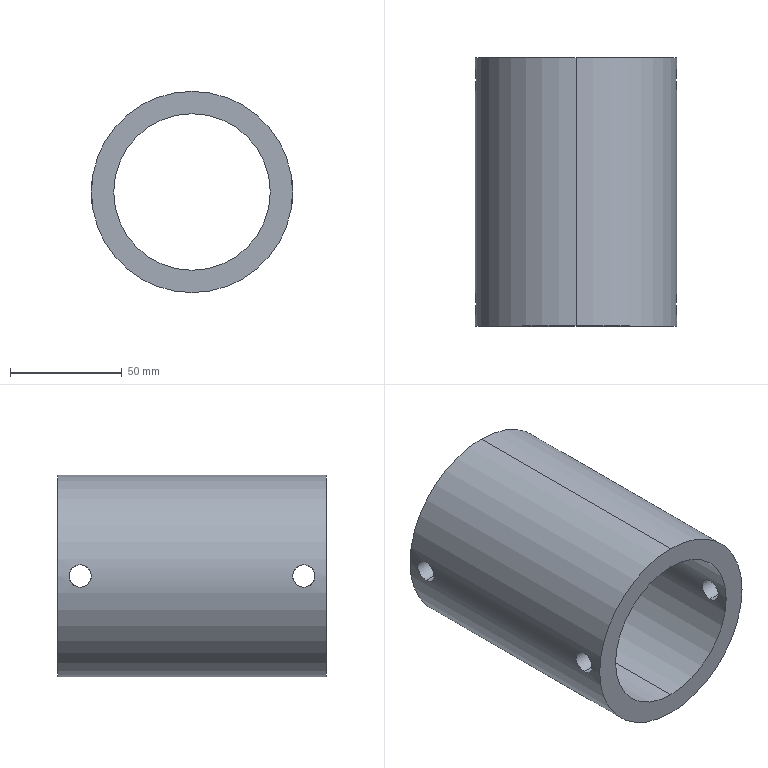Part | SolidWorks | features BaseBody 1 | 1 solid | 14 faces | box 90 x 120 x 90 mm | volume 298445 mm3 | cylinder 12 | plane 2 | commonest cylinder face diameters 10 x8 70 x2 90 x2
STEP:
#1=CARTESIAN_POINT('',(44.721,-50.,5.));
#2=VERTEX_POINT('',#1);
#3=CARTESIAN_POINT('',(44.721,-50.,-5.));
#4=VERTEX_POINT('',#3);
#5=CARTESIAN_POINT('',(44.721,-50.,5.));
#6=CARTESIAN_POINT('',(44.721,-50.33,5.));
#7=CARTESIAN_POINT('',(44.725,-50.656,4.968));
#8=CARTESIAN_POINT('',(44.735,-51.135,4.872));
#9=CARTESIAN_POINT('',(44.74,-51.294,4.833));
#10=CARTESIAN_POINT('',(44.75,-51.608,4.737));
#11=CARTESIAN_POINT('',(44.756,-51.764,4.681));
#12=CARTESIAN_POINT('',(44.775,-52.218,4.493));
#13=CARTESIAN_POINT('',(44.791,-52.505,4.34));
#14=CARTESIAN_POINT('',(44.824,-53.048,3.977));
#15=CARTESIAN_POINT('',(44.843,-53.305,3.766));
#16=CARTESIAN_POINT('',(44.879,-53.766,3.305));
#17=CARTESIAN_POINT('',(44.897,-53.973,3.053));
#18=CARTESIAN_POINT('',(44.931,-54.338,2.507));
#19=CARTESIAN_POINT('',(44.946,-54.494,2.217));
#20=CARTESIAN_POINT('',(44.972,-54.743,1.615));
#21=CARTESIAN_POINT('',(44.982,-54.839,1.3));
#22=CARTESIAN_POINT('',(44.996,-54.968,0.6537));
#23=CARTESIAN_POINT('',(45.,-55.,0.3268));
#24=CARTESIAN_POINT('',(45.,-55.,-0.3342));
#25=CARTESIAN_POINT('',(44.996,-54.967,-0.6592));
#26=CARTESIAN_POINT('',(44.986,-54.871,-1.139));
#27=CARTESIAN_POINT('',(44.982,-54.832,-1.297));
#28=CARTESIAN_POINT('',(44.971,-54.736,-1.611));
#29=CARTESIAN_POINT('',(44.966,-54.68,-1.767));
#30=CARTESIAN_POINT('',(44.946,-54.492,-2.221));
#31=CARTESIAN_POINT('',(44.931,-54.338,-2.508));
#32=CARTESIAN_POINT('',(44.897,-53.975,-3.051));
#33=CARTESIAN_POINT('',(44.879,-53.763,-3.308));
#34=CARTESIAN_POINT('',(44.843,-53.302,-3.768));
#35=CARTESIAN_POINT('',(44.824,-53.051,-3.975));
#36=CARTESIAN_POINT('',(44.791,-52.504,-4.34));
#37=CARTESIAN_POINT('',(44.775,-52.213,-4.495));
#38=CARTESIAN_POINT('',(44.749,-51.612,-4.744));
#39=CARTESIAN_POINT('',(44.739,-51.296,-4.84));
#40=CARTESIAN_POINT('',(44.725,-50.651,-4.968));
#41=CARTESIAN_POINT('',(44.721,-50.326,-5.));
#42=CARTESIAN_POINT('',(44.721,-50.,-5.));
#43=B_SPLINE_CURVE_WITH_KNOTS('',3,(#5,#6,#7,#8,#9,#10,#11,#12,#13,#14,#15,#16,#17,#18,#19,#20,#21,#22,#23,#24,#25,#26,#27,#28,#29,#30,#31,#32,#33,#34,#35,#36,#37,#38,#39,#40,#41,#42),.UNSPECIFIED.,.F.,.F.,(4,2,2,2,2,2,2,2,2,2,2,2,2,2,2,2,2,2,4),(0.02347,0.02445,0.02493,0.02542,0.0264,0.02738,0.02836,0.02933,0.03031,0.03129,0.03227,0.03275,0.03324,0.03422,0.0352,0.03618,0.03715,0.03813,0.03911),.UNSPECIFIED.);
#44=EDGE_CURVE('',#2,#4,#43,.T.);
#45=ORIENTED_EDGE('',*,*,#44,.T.);
#46=CARTESIAN_POINT('',(34.641,-50.,-5.));
#47=VERTEX_POINT('',#46);
#48=CARTESIAN_POINT('',(45.,-50.,-5.));
#49=DIRECTION('',(-1.,0.,0.));
#50=VECTOR('',#49,1000.);
#51=LINE('',#48,#50);
#52=EDGE_CURVE('',#4,#47,#51,.T.);
#53=ORIENTED_EDGE('',*,*,#52,.T.);
#54=CARTESIAN_POINT('',(34.641,-50.,5.));
#55=VERTEX_POINT('',#54);
#56=CARTESIAN_POINT('',(34.641,-50.,5.));
#57=CARTESIAN_POINT('',(34.641,-50.331,5.));
#58=CARTESIAN_POINT('',(34.646,-50.656,4.967));
#59=CARTESIAN_POINT('',(34.659,-51.136,4.872));
#60=CARTESIAN_POINT('',(34.665,-51.294,4.832));
#61=CARTESIAN_POINT('',(34.678,-51.609,4.737));
#62=CARTESIAN_POINT('',(34.686,-51.765,4.681));
#63=CARTESIAN_POINT('',(34.711,-52.219,4.493));
#64=CARTESIAN_POINT('',(34.73,-52.506,4.339));
#65=CARTESIAN_POINT('',(34.774,-53.049,3.976));
#66=CARTESIAN_POINT('',(34.798,-53.306,3.765));
#67=CARTESIAN_POINT('',(34.844,-53.767,3.304));
#68=CARTESIAN_POINT('',(34.868,-53.973,3.053));
#69=CARTESIAN_POINT('',(34.911,-54.339,2.506));
#70=CARTESIAN_POINT('',(34.931,-54.494,2.216));
#71=CARTESIAN_POINT('',(34.964,-54.743,1.614));
#72=CARTESIAN_POINT('',(34.977,-54.84,1.299));
#73=CARTESIAN_POINT('',(34.995,-54.968,0.6532));
#74=CARTESIAN_POINT('',(35.,-55.,0.3284));
#75=CARTESIAN_POINT('',(35.,-55.,-0.3247));
#76=CARTESIAN_POINT('',(34.995,-54.967,-0.6565));
#77=CARTESIAN_POINT('',(34.977,-54.84,-1.298));
#78=CARTESIAN_POINT('',(34.964,-54.745,-1.61));
#79=CARTESIAN_POINT('',(34.939,-54.557,-2.064));
#80=CARTESIAN_POINT('',(34.93,-54.486,-2.214));
#81=CARTESIAN_POINT('',(34.911,-54.331,-2.504));
#82=CARTESIAN_POINT('',(34.9,-54.247,-2.643));
#83=CARTESIAN_POINT('',(34.868,-53.976,-3.049));
#84=CARTESIAN_POINT('',(34.845,-53.769,-3.302));
#85=CARTESIAN_POINT('',(34.797,-53.303,-3.768));
#86=CARTESIAN_POINT('',(34.774,-53.051,-3.975));
#87=CARTESIAN_POINT('',(34.731,-52.509,-4.337));
#88=CARTESIAN_POINT('',(34.711,-52.217,-4.494));
#89=CARTESIAN_POINT('',(34.677,-51.612,-4.744));
#90=CARTESIAN_POINT('',(34.664,-51.3,-4.839));
#91=CARTESIAN_POINT('',(34.646,-50.658,-4.967));
#92=CARTESIAN_POINT('',(34.641,-50.327,-5.));
#93=CARTESIAN_POINT('',(34.641,-50.,-5.));
#94=B_SPLINE_CURVE_WITH_KNOTS('',3,(#56,#57,#58,#59,#60,#61,#62,#63,#64,#65,#66,#67,#68,#69,#70,#71,#72,#73,#74,#75,#76,#77,#78,#79,#80,#81,#82,#83,#84,#85,#86,#87,#88,#89,#90,#91,#92,#93),.UNSPECIFIED.,.F.,.F.,(4,2,2,2,2,2,2,2,2,2,2,2,2,2,2,2,2,2,4),(0.,0.0009783,0.001467,0.001957,0.002935,0.003913,0.004891,0.00587,0.006848,0.007826,0.008804,0.009783,0.01027,0.01076,0.01174,0.01272,0.0137,0.01467,0.01565),.UNSPECIFIED.);
#95=EDGE_CURVE('',#55,#47,#94,.T.);
#96=ORIENTED_EDGE('',*,*,#95,.F.);
#97=CARTESIAN_POINT('',(45.,-50.,5.));
#98=DIRECTION('',(-1.,0.,0.));
#99=VECTOR('',#98,1000.);
#100=LINE('',#97,#99);
#101=EDGE_CURVE('',#2,#55,#100,.T.);
#102=ORIENTED_EDGE('',*,*,#101,.F.);
#103=EDGE_LOOP('',(#45,#53,#96,#102));
#104=FACE_OUTER_BOUND('',#103,.T.);
#105=CARTESIAN_POINT('',(45.,-50.,0.));
#106=DIRECTION('',(-1.,0.,0.));
#107=DIRECTION('',(0.,0.,1.));
#108=AXIS2_PLACEMENT_3D('',#105,#106,#107);
#109=CYLINDRICAL_SURFACE('',#108,5.);
#110=ADVANCED_FACE('',(#104),#109,.F.);
#111=CARTESIAN_POINT('',(-34.641,-50.,-5.));
#112=VERTEX_POINT('',#111);
#113=CARTESIAN_POINT('',(-34.641,-50.,5.));
#114=VERTEX_POINT('',#113);
#115=CARTESIAN_POINT('',(-34.641,-50.,-5.));
#116=CARTESIAN_POINT('',(-34.641,-50.326,-5.));
#117=CARTESIAN_POINT('',(-34.646,-50.651,-4.968));
#118=CARTESIAN_POINT('',(-34.664,-51.297,-4.84));
#119=CARTESIAN_POINT('',(-34.677,-51.612,-4.744));
#120=CARTESIAN_POINT('',(-34.71,-52.214,-4.495));
#121=CARTESIAN_POINT('',(-34.73,-52.505,-4.339));
#122=CARTESIAN_POINT('',(-34.774,-53.051,-3.975));
#123=CARTESIAN_POINT('',(-34.797,-53.303,-3.768));
#124=CARTESIAN_POINT('',(-34.844,-53.764,-3.308));
#125=CARTESIAN_POINT('',(-34.868,-53.975,-3.051));
#126=CARTESIAN_POINT('',(-34.911,-54.338,-2.508));
#127=CARTESIAN_POINT('',(-34.931,-54.491,-2.222));
#128=CARTESIAN_POINT('',(-34.956,-54.68,-1.767));
#129=CARTESIAN_POINT('',(-34.963,-54.736,-1.611));
#130=CARTESIAN_POINT('',(-34.976,-54.832,-1.297));
#131=CARTESIAN_POINT('',(-34.982,-54.871,-1.139));
#132=CARTESIAN_POINT('',(-34.995,-54.967,-0.6595));
#133=CARTESIAN_POINT('',(-35.,-55.,-0.3338));
#134=CARTESIAN_POINT('',(-35.,-55.,0.3271));
#135=CARTESIAN_POINT('',(-34.995,-54.968,0.6522));
#136=CARTESIAN_POINT('',(-34.978,-54.841,1.292));
#137=CARTESIAN_POINT('',(-34.964,-54.745,1.61));
#138=CARTESIAN_POINT('',(-34.931,-54.494,2.215));
#139=CARTESIAN_POINT('',(-34.912,-54.341,2.502));
#140=CARTESIAN_POINT('',(-34.868,-53.979,3.046));
#141=CARTESIAN_POINT('',(-34.845,-53.768,3.303));
#142=CARTESIAN_POINT('',(-34.798,-53.308,3.764));
#143=CARTESIAN_POINT('',(-34.775,-53.057,3.971));
#144=CARTESIAN_POINT('',(-34.731,-52.51,4.337));
#145=CARTESIAN_POINT('',(-34.711,-52.22,4.492));
#146=CARTESIAN_POINT('',(-34.678,-51.619,4.742));
#147=CARTESIAN_POINT('',(-34.664,-51.304,4.838));
#148=CARTESIAN_POINT('',(-34.646,-50.658,4.968));
#149=CARTESIAN_POINT('',(-34.641,-50.331,5.));
#150=CARTESIAN_POINT('',(-34.641,-50.,5.));
#151=B_SPLINE_CURVE_WITH_KNOTS('',3,(#115,#116,#117,#118,#119,#120,#121,#122,#123,#124,#125,#126,#127,#128,#129,#130,#131,#132,#133,#134,#135,#136,#137,#138,#139,#140,#141,#142,#143,#144,#145,#146,#147,#148,#149,#150),.UNSPECIFIED.,.F.,.F.,(4,2,2,2,2,2,2,2,2,2,2,2,2,2,2,2,2,4),(0.01565,0.01663,0.01761,0.01859,0.01956,0.02054,0.02152,0.02201,0.0225,0.02348,0.02445,0.02543,0.02641,0.02739,0.02837,0.02934,0.03032,0.0313),.UNSPECIFIED.);
#152=EDGE_CURVE('',#112,#114,#151,.T.);
#153=ORIENTED_EDGE('',*,*,#152,.F.);
#154=CARTESIAN_POINT('',(-44.721,-50.,-5.));
#155=VERTEX_POINT('',#154);
#156=CARTESIAN_POINT('',(45.,-50.,-5.));
#157=DIRECTION('',(-1.,0.,0.));
#158=VECTOR('',#157,1000.);
#159=LINE('',#156,#158);
#160=EDGE_CURVE('',#112,#155,#159,.T.);
#161=ORIENTED_EDGE('',*,*,#160,.T.);
#162=CARTESIAN_POINT('',(-44.721,-50.,5.));
#163=VERTEX_POINT('',#162);
#164=CARTESIAN_POINT('',(-44.721,-50.,-5.));
#165=CARTESIAN_POINT('',(-44.721,-50.326,-5.));
#166=CARTESIAN_POINT('',(-44.725,-50.651,-4.968));
#167=CARTESIAN_POINT('',(-44.739,-51.296,-4.84));
#168=CARTESIAN_POINT('',(-44.749,-51.612,-4.744));
#169=CARTESIAN_POINT('',(-44.775,-52.214,-4.495));
#170=CARTESIAN_POINT('',(-44.791,-52.504,-4.34));
#171=CARTESIAN_POINT('',(-44.824,-53.051,-3.975));
#172=CARTESIAN_POINT('',(-44.843,-53.303,-3.768));
#173=CARTESIAN_POINT('',(-44.879,-53.764,-3.308));
#174=CARTESIAN_POINT('',(-44.897,-53.975,-3.051));
#175=CARTESIAN_POINT('',(-44.931,-54.338,-2.508));
#176=CARTESIAN_POINT('',(-44.946,-54.492,-2.221));
#177=CARTESIAN_POINT('',(-44.966,-54.68,-1.767));
#178=CARTESIAN_POINT('',(-44.971,-54.736,-1.611));
#179=CARTESIAN_POINT('',(-44.982,-54.832,-1.297));
#180=CARTESIAN_POINT('',(-44.986,-54.871,-1.138));
#181=CARTESIAN_POINT('',(-44.996,-54.967,-0.6591));
#182=CARTESIAN_POINT('',(-45.,-55.,-0.3342));
#183=CARTESIAN_POINT('',(-45.,-55.,0.3267));
#184=CARTESIAN_POINT('',(-44.996,-54.968,0.652));
#185=CARTESIAN_POINT('',(-44.986,-54.873,1.132));
#186=CARTESIAN_POINT('',(-44.982,-54.834,1.29));
#187=CARTESIAN_POINT('',(-44.972,-54.738,1.604));
#188=CARTESIAN_POINT('',(-44.966,-54.683,1.76));
#189=CARTESIAN_POINT('',(-44.946,-54.495,2.215));
#190=CARTESIAN_POINT('',(-44.931,-54.341,2.502));
#191=CARTESIAN_POINT('',(-44.898,-53.979,3.045));
#192=CARTESIAN_POINT('',(-44.879,-53.768,3.303));
#193=CARTESIAN_POINT('',(-44.843,-53.308,3.764));
#194=CARTESIAN_POINT('',(-44.825,-53.056,3.971));
#195=CARTESIAN_POINT('',(-44.791,-52.51,4.337));
#196=CARTESIAN_POINT('',(-44.775,-52.22,4.492));
#197=CARTESIAN_POINT('',(-44.75,-51.619,4.742));
#198=CARTESIAN_POINT('',(-44.739,-51.304,4.838));
#199=CARTESIAN_POINT('',(-44.725,-50.657,4.968));
#200=CARTESIAN_POINT('',(-44.721,-50.331,5.));
#201=CARTESIAN_POINT('',(-44.721,-50.,5.));
#202=B_SPLINE_CURVE_WITH_KNOTS('',3,(#164,#165,#166,#167,#168,#169,#170,#171,#172,#173,#174,#175,#176,#177,#178,#179,#180,#181,#182,#183,#184,#185,#186,#187,#188,#189,#190,#191,#192,#193,#194,#195,#196,#197,#198,#199,#200,#201),.UNSPECIFIED.,.F.,.F.,(4,2,2,2,2,2,2,2,2,2,2,2,2,2,2,2,2,2,4),(0.01564,0.01662,0.0176,0.01858,0.01955,0.02053,0.02151,0.022,0.02249,0.02346,0.02444,0.02493,0.02542,0.0264,0.02737,0.02835,0.02933,0.03031,0.03128),.UNSPECIFIED.);
#203=EDGE_CURVE('',#155,#163,#202,.T.);
#204=ORIENTED_EDGE('',*,*,#203,.T.);
#205=CARTESIAN_POINT('',(45.,-50.,5.));
#206=DIRECTION('',(-1.,0.,0.));
#207=VECTOR('',#206,1000.);
#208=LINE('',#205,#207);
#209=EDGE_CURVE('',#114,#163,#208,.T.);
#210=ORIENTED_EDGE('',*,*,#209,.F.);
#211=EDGE_LOOP('',(#153,#161,#204,#210));
#212=FACE_OUTER_BOUND('',#211,.T.);
#213=CARTESIAN_POINT('',(45.,-50.,0.));
#214=DIRECTION('',(-1.,0.,0.));
#215=DIRECTION('',(0.,0.,1.));
#216=AXIS2_PLACEMENT_3D('',#213,#214,#215);
#217=CYLINDRICAL_SURFACE('',#216,5.);
#218=ADVANCED_FACE('',(#212),#217,.F.);
#219=CARTESIAN_POINT('',(44.721,50.,-5.));
#220=VERTEX_POINT('',#219);
#221=CARTESIAN_POINT('',(44.721,50.,5.));
#222=VERTEX_POINT('',#221);
#223=CARTESIAN_POINT('',(44.721,50.,-5.));
#224=CARTESIAN_POINT('',(44.721,49.67,-5.));
#225=CARTESIAN_POINT('',(44.725,49.344,-4.968));
#226=CARTESIAN_POINT('',(44.735,48.865,-4.872));
#227=CARTESIAN_POINT('',(44.74,48.706,-4.833));
#228=CARTESIAN_POINT('',(44.75,48.392,-4.737));
#229=CARTESIAN_POINT('',(44.756,48.236,-4.681));
#230=CARTESIAN_POINT('',(44.775,47.782,-4.493));
#231=CARTESIAN_POINT('',(44.791,47.495,-4.34));
#232=CARTESIAN_POINT('',(44.824,46.952,-3.977));
#233=CARTESIAN_POINT('',(44.843,46.695,-3.766));
#234=CARTESIAN_POINT('',(44.879,46.234,-3.305));
#235=CARTESIAN_POINT('',(44.897,46.027,-3.053));
#236=CARTESIAN_POINT('',(44.931,45.662,-2.507));
#237=CARTESIAN_POINT('',(44.946,45.506,-2.217));
#238=CARTESIAN_POINT('',(44.972,45.257,-1.615));
#239=CARTESIAN_POINT('',(44.982,45.161,-1.3));
#240=CARTESIAN_POINT('',(44.996,45.032,-0.6537));
#241=CARTESIAN_POINT('',(45.,45.,-0.3268));
#242=CARTESIAN_POINT('',(45.,45.,0.3342));
#243=CARTESIAN_POINT('',(44.996,45.033,0.6592));
#244=CARTESIAN_POINT('',(44.986,45.129,1.139));
#245=CARTESIAN_POINT('',(44.982,45.168,1.297));
#246=CARTESIAN_POINT('',(44.971,45.264,1.611));
#247=CARTESIAN_POINT('',(44.966,45.32,1.767));
#248=CARTESIAN_POINT('',(44.946,45.508,2.221));
#249=CARTESIAN_POINT('',(44.931,45.662,2.508));
#250=CARTESIAN_POINT('',(44.897,46.025,3.051));
#251=CARTESIAN_POINT('',(44.879,46.237,3.308));
#252=CARTESIAN_POINT('',(44.843,46.698,3.768));
#253=CARTESIAN_POINT('',(44.824,46.949,3.975));
#254=CARTESIAN_POINT('',(44.791,47.496,4.34));
#255=CARTESIAN_POINT('',(44.775,47.787,4.495));
#256=CARTESIAN_POINT('',(44.749,48.388,4.744));
#257=CARTESIAN_POINT('',(44.739,48.704,4.84));
#258=CARTESIAN_POINT('',(44.725,49.349,4.968));
#259=CARTESIAN_POINT('',(44.721,49.674,5.));
#260=CARTESIAN_POINT('',(44.721,50.,5.));
#261=B_SPLINE_CURVE_WITH_KNOTS('',3,(#223,#224,#225,#226,#227,#228,#229,#230,#231,#232,#233,#234,#235,#236,#237,#238,#239,#240,#241,#242,#243,#244,#245,#246,#247,#248,#249,#250,#251,#252,#253,#254,#255,#256,#257,#258,#259,#260),.UNSPECIFIED.,.F.,.F.,(4,2,2,2,2,2,2,2,2,2,2,2,2,2,2,2,2,2,4),(0.02347,0.02445,0.02493,0.02542,0.0264,0.02738,0.02836,0.02933,0.03031,0.03129,0.03227,0.03275,0.03324,0.03422,0.0352,0.03618,0.03715,0.03813,0.03911),.UNSPECIFIED.);
#262=EDGE_CURVE('',#220,#222,#261,.T.);
#263=ORIENTED_EDGE('',*,*,#262,.F.);
#264=CARTESIAN_POINT('',(34.641,50.,-5.));
#265=VERTEX_POINT('',#264);
#266=CARTESIAN_POINT('',(45.,50.,-5.));
#267=DIRECTION('',(-1.,0.,0.));
#268=VECTOR('',#267,1000.);
#269=LINE('',#266,#268);
#270=EDGE_CURVE('',#220,#265,#269,.T.);
#271=ORIENTED_EDGE('',*,*,#270,.T.);
#272=CARTESIAN_POINT('',(34.641,50.,5.));
#273=VERTEX_POINT('',#272);
#274=CARTESIAN_POINT('',(34.641,50.,-5.));
#275=CARTESIAN_POINT('',(34.641,49.674,-5.));
#276=CARTESIAN_POINT('',(34.646,49.349,-4.968));
#277=CARTESIAN_POINT('',(34.664,48.703,-4.84));
#278=CARTESIAN_POINT('',(34.677,48.388,-4.744));
#279=CARTESIAN_POINT('',(34.71,47.786,-4.495));
#280=CARTESIAN_POINT('',(34.73,47.495,-4.339));
#281=CARTESIAN_POINT('',(34.774,46.949,-3.975));
#282=CARTESIAN_POINT('',(34.797,46.697,-3.768));
#283=CARTESIAN_POINT('',(34.844,46.236,-3.308));
#284=CARTESIAN_POINT('',(34.868,46.025,-3.051));
#285=CARTESIAN_POINT('',(34.911,45.662,-2.508));
#286=CARTESIAN_POINT('',(34.931,45.509,-2.222));
#287=CARTESIAN_POINT('',(34.956,45.32,-1.767));
#288=CARTESIAN_POINT('',(34.963,45.264,-1.611));
#289=CARTESIAN_POINT('',(34.976,45.168,-1.297));
#290=CARTESIAN_POINT('',(34.982,45.129,-1.139));
#291=CARTESIAN_POINT('',(34.995,45.033,-0.6595));
#292=CARTESIAN_POINT('',(35.,45.,-0.3338));
#293=CARTESIAN_POINT('',(35.,45.,0.3271));
#294=CARTESIAN_POINT('',(34.995,45.032,0.6522));
#295=CARTESIAN_POINT('',(34.978,45.159,1.292));
#296=CARTESIAN_POINT('',(34.964,45.255,1.61));
#297=CARTESIAN_POINT('',(34.931,45.506,2.215));
#298=CARTESIAN_POINT('',(34.912,45.659,2.502));
#299=CARTESIAN_POINT('',(34.868,46.021,3.046));
#300=CARTESIAN_POINT('',(34.845,46.232,3.303));
#301=CARTESIAN_POINT('',(34.798,46.692,3.764));
#302=CARTESIAN_POINT('',(34.775,46.943,3.971));
#303=CARTESIAN_POINT('',(34.731,47.49,4.337));
#304=CARTESIAN_POINT('',(34.711,47.78,4.492));
#305=CARTESIAN_POINT('',(34.678,48.381,4.742));
#306=CARTESIAN_POINT('',(34.664,48.696,4.838));
#307=CARTESIAN_POINT('',(34.646,49.342,4.968));
#308=CARTESIAN_POINT('',(34.641,49.669,5.));
#309=CARTESIAN_POINT('',(34.641,50.,5.));
#310=B_SPLINE_CURVE_WITH_KNOTS('',3,(#274,#275,#276,#277,#278,#279,#280,#281,#282,#283,#284,#285,#286,#287,#288,#289,#290,#291,#292,#293,#294,#295,#296,#297,#298,#299,#300,#301,#302,#303,#304,#305,#306,#307,#308,#309),.UNSPECIFIED.,.F.,.F.,(4,2,2,2,2,2,2,2,2,2,2,2,2,2,2,2,2,4),(0.01565,0.01663,0.01761,0.01859,0.01956,0.02054,0.02152,0.02201,0.0225,0.02348,0.02445,0.02543,0.02641,0.02739,0.02837,0.02934,0.03032,0.0313),.UNSPECIFIED.);
#311=EDGE_CURVE('',#265,#273,#310,.T.);
#312=ORIENTED_EDGE('',*,*,#311,.T.);
#313=CARTESIAN_POINT('',(45.,50.,5.));
#314=DIRECTION('',(-1.,0.,0.));
#315=VECTOR('',#314,1000.);
#316=LINE('',#313,#315);
#317=EDGE_CURVE('',#222,#273,#316,.T.);
#318=ORIENTED_EDGE('',*,*,#317,.F.);
#319=EDGE_LOOP('',(#263,#271,#312,#318));
#320=FACE_OUTER_BOUND('',#319,.T.);
#321=CARTESIAN_POINT('',(45.,50.,0.));
#322=DIRECTION('',(-1.,0.,0.));
#323=DIRECTION('',(0.,0.,1.));
#324=AXIS2_PLACEMENT_3D('',#321,#322,#323);
#325=CYLINDRICAL_SURFACE('',#324,5.);
#326=ADVANCED_FACE('',(#320),#325,.F.);
#327=CARTESIAN_POINT('',(-34.641,50.,5.));
#328=VERTEX_POINT('',#327);
#329=CARTESIAN_POINT('',(-34.641,50.,-5.));
#330=VERTEX_POINT('',#329);
#331=CARTESIAN_POINT('',(-34.641,50.,5.));
#332=CARTESIAN_POINT('',(-34.641,49.669,5.));
#333=CARTESIAN_POINT('',(-34.646,49.344,4.967));
#334=CARTESIAN_POINT('',(-34.659,48.864,4.872));
#335=CARTESIAN_POINT('',(-34.665,48.706,4.832));
#336=CARTESIAN_POINT('',(-34.678,48.391,4.737));
#337=CARTESIAN_POINT('',(-34.686,48.235,4.681));
#338=CARTESIAN_POINT('',(-34.711,47.781,4.493));
#339=CARTESIAN_POINT('',(-34.73,47.494,4.339));
#340=CARTESIAN_POINT('',(-34.774,46.951,3.976));
#341=CARTESIAN_POINT('',(-34.798,46.694,3.765));
#342=CARTESIAN_POINT('',(-34.844,46.233,3.304));
#343=CARTESIAN_POINT('',(-34.868,46.027,3.053));
#344=CARTESIAN_POINT('',(-34.911,45.661,2.506));
#345=CARTESIAN_POINT('',(-34.931,45.506,2.216));
#346=CARTESIAN_POINT('',(-34.964,45.257,1.614));
#347=CARTESIAN_POINT('',(-34.977,45.16,1.299));
#348=CARTESIAN_POINT('',(-34.995,45.032,0.6532));
#349=CARTESIAN_POINT('',(-35.,45.,0.3284));
#350=CARTESIAN_POINT('',(-35.,45.,-0.3247));
#351=CARTESIAN_POINT('',(-34.995,45.033,-0.6565));
#352=CARTESIAN_POINT('',(-34.977,45.16,-1.298));
#353=CARTESIAN_POINT('',(-34.964,45.255,-1.61));
#354=CARTESIAN_POINT('',(-34.939,45.443,-2.064));
#355=CARTESIAN_POINT('',(-34.93,45.514,-2.214));
#356=CARTESIAN_POINT('',(-34.911,45.669,-2.504));
#357=CARTESIAN_POINT('',(-34.9,45.753,-2.643));
#358=CARTESIAN_POINT('',(-34.868,46.024,-3.049));
#359=CARTESIAN_POINT('',(-34.845,46.231,-3.302));
#360=CARTESIAN_POINT('',(-34.797,46.697,-3.768));
#361=CARTESIAN_POINT('',(-34.774,46.949,-3.975));
#362=CARTESIAN_POINT('',(-34.731,47.491,-4.337));
#363=CARTESIAN_POINT('',(-34.711,47.783,-4.494));
#364=CARTESIAN_POINT('',(-34.677,48.388,-4.744));
#365=CARTESIAN_POINT('',(-34.664,48.7,-4.839));
#366=CARTESIAN_POINT('',(-34.646,49.342,-4.967));
#367=CARTESIAN_POINT('',(-34.641,49.673,-5.));
#368=CARTESIAN_POINT('',(-34.641,50.,-5.));
#369=B_SPLINE_CURVE_WITH_KNOTS('',3,(#331,#332,#333,#334,#335,#336,#337,#338,#339,#340,#341,#342,#343,#344,#345,#346,#347,#348,#349,#350,#351,#352,#353,#354,#355,#356,#357,#358,#359,#360,#361,#362,#363,#364,#365,#366,#367,#368),.UNSPECIFIED.,.F.,.F.,(4,2,2,2,2,2,2,2,2,2,2,2,2,2,2,2,2,2,4),(0.,0.0009783,0.001467,0.001957,0.002935,0.003913,0.004891,0.00587,0.006848,0.007826,0.008804,0.009783,0.01027,0.01076,0.01174,0.01272,0.0137,0.01467,0.01565),.UNSPECIFIED.);
#370=EDGE_CURVE('',#328,#330,#369,.T.);
#371=ORIENTED_EDGE('',*,*,#370,.T.);
#372=CARTESIAN_POINT('',(-44.721,50.,-5.));
#373=VERTEX_POINT('',#372);
#374=CARTESIAN_POINT('',(45.,50.,-5.));
#375=DIRECTION('',(-1.,0.,0.));
#376=VECTOR('',#375,1000.);
#377=LINE('',#374,#376);
#378=EDGE_CURVE('',#330,#373,#377,.T.);
#379=ORIENTED_EDGE('',*,*,#378,.T.);
#380=CARTESIAN_POINT('',(-44.721,50.,5.));
#381=VERTEX_POINT('',#380);
#382=CARTESIAN_POINT('',(-44.721,50.,5.));
#383=CARTESIAN_POINT('',(-44.721,49.669,5.));
#384=CARTESIAN_POINT('',(-44.725,49.344,4.968));
#385=CARTESIAN_POINT('',(-44.735,48.865,4.872));
#386=CARTESIAN_POINT('',(-44.74,48.706,4.833));
#387=CARTESIAN_POINT('',(-44.75,48.392,4.737));
#388=CARTESIAN_POINT('',(-44.756,48.236,4.681));
#389=CARTESIAN_POINT('',(-44.775,47.782,4.493));
#390=CARTESIAN_POINT('',(-44.791,47.495,4.339));
#391=CARTESIAN_POINT('',(-44.824,46.951,3.976));
#392=CARTESIAN_POINT('',(-44.843,46.694,3.765));
#393=CARTESIAN_POINT('',(-44.879,46.233,3.304));
#394=CARTESIAN_POINT('',(-44.897,46.026,3.053));
#395=CARTESIAN_POINT('',(-44.931,45.661,2.506));
#396=CARTESIAN_POINT('',(-44.946,45.506,2.215));
#397=CARTESIAN_POINT('',(-44.972,45.256,1.614));
#398=CARTESIAN_POINT('',(-44.982,45.16,1.298));
#399=CARTESIAN_POINT('',(-44.996,45.032,0.6528));
#400=CARTESIAN_POINT('',(-45.,45.,0.3282));
#401=CARTESIAN_POINT('',(-45.,45.,-0.3246));
#402=CARTESIAN_POINT('',(-44.996,45.032,-0.6561));
#403=CARTESIAN_POINT('',(-44.982,45.16,-1.298));
#404=CARTESIAN_POINT('',(-44.972,45.255,-1.609));
#405=CARTESIAN_POINT('',(-44.953,45.443,-2.064));
#406=CARTESIAN_POINT('',(-44.946,45.514,-2.214));
#407=CARTESIAN_POINT('',(-44.931,45.668,-2.503));
#408=CARTESIAN_POINT('',(-44.923,45.753,-2.643));
#409=CARTESIAN_POINT('',(-44.897,46.024,-3.049));
#410=CARTESIAN_POINT('',(-44.879,46.231,-3.302));
#411=CARTESIAN_POINT('',(-44.843,46.697,-3.768));
#412=CARTESIAN_POINT('',(-44.824,46.95,-3.975));
#413=CARTESIAN_POINT('',(-44.799,47.356,-4.247));
#414=CARTESIAN_POINT('',(-44.791,47.496,-4.331));
#415=CARTESIAN_POINT('',(-44.776,47.785,-4.486));
#416=CARTESIAN_POINT('',(-44.769,47.935,-4.557));
#417=CARTESIAN_POINT('',(-44.749,48.389,-4.745));
#418=CARTESIAN_POINT('',(-44.739,48.701,-4.839));
#419=CARTESIAN_POINT('',(-44.725,49.342,-4.967));
#420=CARTESIAN_POINT('',(-44.721,49.674,-5.));
#421=CARTESIAN_POINT('',(-44.721,50.,-5.));
#422=B_SPLINE_CURVE_WITH_KNOTS('',3,(#382,#383,#384,#385,#386,#387,#388,#389,#390,#391,#392,#393,#394,#395,#396,#397,#398,#399,#400,#401,#402,#403,#404,#405,#406,#407,#408,#409,#410,#411,#412,#413,#414,#415,#416,#417,#418,#419,#420,#421),.UNSPECIFIED.,.F.,.F.,(4,2,2,2,2,2,2,2,2,2,2,2,2,2,2,2,2,2,2,4),(0.,0.0009778,0.001467,0.001956,0.002933,0.003911,0.004889,0.005867,0.006844,0.007822,0.0088,0.009778,0.01027,0.01076,0.01173,0.01271,0.0132,0.01369,0.01467,0.01564),.UNSPECIFIED.);
#423=EDGE_CURVE('',#381,#373,#422,.T.);
#424=ORIENTED_EDGE('',*,*,#423,.F.);
#425=CARTESIAN_POINT('',(45.,50.,5.));
#426=DIRECTION('',(-1.,0.,0.));
#427=VECTOR('',#426,1000.);
#428=LINE('',#425,#427);
#429=EDGE_CURVE('',#328,#381,#428,.T.);
#430=ORIENTED_EDGE('',*,*,#429,.F.);
#431=EDGE_LOOP('',(#371,#379,#424,#430));
#432=FACE_OUTER_BOUND('',#431,.T.);
#433=CARTESIAN_POINT('',(45.,50.,0.));
#434=DIRECTION('',(-1.,0.,0.));
#435=DIRECTION('',(0.,0.,1.));
#436=AXIS2_PLACEMENT_3D('',#433,#434,#435);
#437=CYLINDRICAL_SURFACE('',#436,5.);
#438=ADVANCED_FACE('',(#432),#437,.F.);
#439=ORIENTED_EDGE('',*,*,#370,.F.);
#440=CARTESIAN_POINT('',(-34.641,50.,-5.));
#441=CARTESIAN_POINT('',(-34.641,50.326,-5.));
#442=CARTESIAN_POINT('',(-34.646,50.651,-4.968));
#443=CARTESIAN_POINT('',(-34.664,51.297,-4.84));
#444=CARTESIAN_POINT('',(-34.677,51.612,-4.744));
#445=CARTESIAN_POINT('',(-34.71,52.214,-4.495));
#446=CARTESIAN_POINT('',(-34.73,52.505,-4.339));
#447=CARTESIAN_POINT('',(-34.774,53.051,-3.975));
#448=CARTESIAN_POINT('',(-34.797,53.303,-3.768));
#449=CARTESIAN_POINT('',(-34.844,53.764,-3.308));
#450=CARTESIAN_POINT('',(-34.868,53.975,-3.051));
#451=CARTESIAN_POINT('',(-34.911,54.338,-2.508));
#452=CARTESIAN_POINT('',(-34.931,54.491,-2.222));
#453=CARTESIAN_POINT('',(-34.956,54.68,-1.767));
#454=CARTESIAN_POINT('',(-34.963,54.736,-1.611));
#455=CARTESIAN_POINT('',(-34.976,54.832,-1.297));
#456=CARTESIAN_POINT('',(-34.982,54.871,-1.139));
#457=CARTESIAN_POINT('',(-34.995,54.967,-0.6595));
#458=CARTESIAN_POINT('',(-35.,55.,-0.3338));
#459=CARTESIAN_POINT('',(-35.,55.,0.3271));
#460=CARTESIAN_POINT('',(-34.995,54.968,0.6522));
#461=CARTESIAN_POINT('',(-34.978,54.841,1.292));
#462=CARTESIAN_POINT('',(-34.964,54.745,1.61));
#463=CARTESIAN_POINT('',(-34.931,54.494,2.215));
#464=CARTESIAN_POINT('',(-34.912,54.341,2.502));
#465=CARTESIAN_POINT('',(-34.868,53.979,3.046));
#466=CARTESIAN_POINT('',(-34.845,53.768,3.303));
#467=CARTESIAN_POINT('',(-34.798,53.308,3.764));
#468=CARTESIAN_POINT('',(-34.775,53.057,3.971));
#469=CARTESIAN_POINT('',(-34.731,52.51,4.337));
#470=CARTESIAN_POINT('',(-34.711,52.22,4.492));
#471=CARTESIAN_POINT('',(-34.678,51.619,4.742));
#472=CARTESIAN_POINT('',(-34.664,51.304,4.838));
#473=CARTESIAN_POINT('',(-34.646,50.658,4.968));
#474=CARTESIAN_POINT('',(-34.641,50.331,5.));
#475=CARTESIAN_POINT('',(-34.641,50.,5.));
#476=B_SPLINE_CURVE_WITH_KNOTS('',3,(#440,#441,#442,#443,#444,#445,#446,#447,#448,#449,#450,#451,#452,#453,#454,#455,#456,#457,#458,#459,#460,#461,#462,#463,#464,#465,#466,#467,#468,#469,#470,#471,#472,#473,#474,#475),.UNSPECIFIED.,.F.,.F.,(4,2,2,2,2,2,2,2,2,2,2,2,2,2,2,2,2,4),(0.01565,0.01663,0.01761,0.01859,0.01956,0.02054,0.02152,0.02201,0.0225,0.02348,0.02445,0.02543,0.02641,0.02739,0.02837,0.02934,0.03032,0.0313),.UNSPECIFIED.);
#477=EDGE_CURVE('',#330,#328,#476,.T.);
#478=ORIENTED_EDGE('',*,*,#477,.F.);
#479=EDGE_LOOP('',(#439,#478));
#480=FACE_BOUND('',#479,.T.);
#481=CARTESIAN_POINT('',(-34.641,-50.,5.));
#482=CARTESIAN_POINT('',(-34.641,-49.669,5.));
#483=CARTESIAN_POINT('',(-34.646,-49.344,4.967));
#484=CARTESIAN_POINT('',(-34.659,-48.864,4.872));
#485=CARTESIAN_POINT('',(-34.665,-48.706,4.832));
#486=CARTESIAN_POINT('',(-34.678,-48.391,4.737));
#487=CARTESIAN_POINT('',(-34.686,-48.235,4.681));
#488=CARTESIAN_POINT('',(-34.711,-47.781,4.493));
#489=CARTESIAN_POINT('',(-34.73,-47.494,4.339));
#490=CARTESIAN_POINT('',(-34.774,-46.951,3.976));
#491=CARTESIAN_POINT('',(-34.798,-46.694,3.765));
#492=CARTESIAN_POINT('',(-34.844,-46.233,3.304));
#493=CARTESIAN_POINT('',(-34.868,-46.027,3.053));
#494=CARTESIAN_POINT('',(-34.911,-45.661,2.506));
#495=CARTESIAN_POINT('',(-34.931,-45.506,2.216));
#496=CARTESIAN_POINT('',(-34.964,-45.257,1.614));
#497=CARTESIAN_POINT('',(-34.977,-45.16,1.299));
#498=CARTESIAN_POINT('',(-34.995,-45.032,0.6532));
#499=CARTESIAN_POINT('',(-35.,-45.,0.3284));
#500=CARTESIAN_POINT('',(-35.,-45.,-0.3247));
#501=CARTESIAN_POINT('',(-34.995,-45.033,-0.6565));
#502=CARTESIAN_POINT('',(-34.977,-45.16,-1.298));
#503=CARTESIAN_POINT('',(-34.964,-45.255,-1.61));
#504=CARTESIAN_POINT('',(-34.939,-45.443,-2.064));
#505=CARTESIAN_POINT('',(-34.93,-45.514,-2.214));
#506=CARTESIAN_POINT('',(-34.911,-45.669,-2.504));
#507=CARTESIAN_POINT('',(-34.9,-45.753,-2.643));
#508=CARTESIAN_POINT('',(-34.868,-46.024,-3.049));
#509=CARTESIAN_POINT('',(-34.845,-46.231,-3.302));
#510=CARTESIAN_POINT('',(-34.797,-46.697,-3.768));
#511=CARTESIAN_POINT('',(-34.774,-46.949,-3.975));
#512=CARTESIAN_POINT('',(-34.731,-47.491,-4.337));
#513=CARTESIAN_POINT('',(-34.711,-47.783,-4.494));
#514=CARTESIAN_POINT('',(-34.677,-48.388,-4.744));
#515=CARTESIAN_POINT('',(-34.664,-48.7,-4.839));
#516=CARTESIAN_POINT('',(-34.646,-49.342,-4.967));
#517=CARTESIAN_POINT('',(-34.641,-49.673,-5.));
#518=CARTESIAN_POINT('',(-34.641,-50.,-5.));
#519=B_SPLINE_CURVE_WITH_KNOTS('',3,(#481,#482,#483,#484,#485,#486,#487,#488,#489,#490,#491,#492,#493,#494,#495,#496,#497,#498,#499,#500,#501,#502,#503,#504,#505,#506,#507,#508,#509,#510,#511,#512,#513,#514,#515,#516,#517,#518),.UNSPECIFIED.,.F.,.F.,(4,2,2,2,2,2,2,2,2,2,2,2,2,2,2,2,2,2,4),(0.,0.0009783,0.001467,0.001957,0.002935,0.003913,0.004891,0.00587,0.006848,0.007826,0.008804,0.009783,0.01027,0.01076,0.01174,0.01272,0.0137,0.01467,0.01565),.UNSPECIFIED.);
#520=EDGE_CURVE('',#114,#112,#519,.T.);
#521=ORIENTED_EDGE('',*,*,#520,.T.);
#522=ORIENTED_EDGE('',*,*,#152,.T.);
#523=EDGE_LOOP('',(#521,#522));
#524=FACE_BOUND('',#523,.T.);
#525=CARTESIAN_POINT('',(0.,60.,-35.));
#526=VERTEX_POINT('',#525);
#527=CARTESIAN_POINT('',(0.,60.,35.));
#528=VERTEX_POINT('',#527);
#529=CARTESIAN_POINT('',(0.,60.,0.));
#530=DIRECTION('',(0.,1.,0.));
#531=DIRECTION('',(0.,0.,1.));
#532=AXIS2_PLACEMENT_3D('',#529,#530,#531);
#533=CIRCLE('',#532,35.);
#534=EDGE_CURVE('',#526,#528,#533,.T.);
#535=ORIENTED_EDGE('',*,*,#534,.T.);
#536=CARTESIAN_POINT('',(0.,-60.,35.));
#537=VERTEX_POINT('',#536);
#538=CARTESIAN_POINT('',(0.,60.,35.));
#539=DIRECTION('',(0.,-1.,0.));
#540=VECTOR('',#539,1000.);
#541=LINE('',#538,#540);
#542=EDGE_CURVE('',#528,#537,#541,.T.);
#543=ORIENTED_EDGE('',*,*,#542,.T.);
#544=CARTESIAN_POINT('',(0.,-60.,-35.));
#545=VERTEX_POINT('',#544);
#546=CARTESIAN_POINT('',(0.,-60.,0.));
#547=DIRECTION('',(0.,1.,0.));
#548=DIRECTION('',(0.,0.,1.));
#549=AXIS2_PLACEMENT_3D('',#546,#547,#548);
#550=CIRCLE('',#549,35.);
#551=EDGE_CURVE('',#545,#537,#550,.T.);
#552=ORIENTED_EDGE('',*,*,#551,.F.);
#553=CARTESIAN_POINT('',(0.,60.,-35.));
#554=DIRECTION('',(0.,-1.,0.));
#555=VECTOR('',#554,1000.);
#556=LINE('',#553,#555);
#557=EDGE_CURVE('',#526,#545,#556,.T.);
#558=ORIENTED_EDGE('',*,*,#557,.F.);
#559=EDGE_LOOP('',(#535,#543,#552,#558));
#560=FACE_OUTER_BOUND('',#559,.T.);
#561=CARTESIAN_POINT('',(0.,60.,0.));
#562=DIRECTION('',(0.,-1.,0.));
#563=DIRECTION('',(0.,0.,-1.));
#564=AXIS2_PLACEMENT_3D('',#561,#562,#563);
#565=CYLINDRICAL_SURFACE('',#564,35.);
#566=ADVANCED_FACE('',(#480,#524,#560),#565,.F.);
#567=ORIENTED_EDGE('',*,*,#44,.F.);
#568=CARTESIAN_POINT('',(44.721,-50.,-5.));
#569=CARTESIAN_POINT('',(44.721,-49.674,-5.));
#570=CARTESIAN_POINT('',(44.725,-49.342,-4.967));
#571=CARTESIAN_POINT('',(44.739,-48.701,-4.839));
#572=CARTESIAN_POINT('',(44.749,-48.389,-4.745));
#573=CARTESIAN_POINT('',(44.769,-47.935,-4.556));
#574=CARTESIAN_POINT('',(44.776,-47.785,-4.485));
#575=CARTESIAN_POINT('',(44.791,-47.495,-4.331));
#576=CARTESIAN_POINT('',(44.799,-47.355,-4.247));
#577=CARTESIAN_POINT('',(44.824,-46.949,-3.975));
#578=CARTESIAN_POINT('',(44.843,-46.697,-3.768));
#579=CARTESIAN_POINT('',(44.879,-46.23,-3.301));
#580=CARTESIAN_POINT('',(44.897,-46.024,-3.049));
#581=CARTESIAN_POINT('',(44.923,-45.752,-2.643));
#582=CARTESIAN_POINT('',(44.931,-45.668,-2.503));
#583=CARTESIAN_POINT('',(44.946,-45.514,-2.213));
#584=CARTESIAN_POINT('',(44.953,-45.443,-2.063));
#585=CARTESIAN_POINT('',(44.972,-45.255,-1.609));
#586=CARTESIAN_POINT('',(44.982,-45.16,-1.298));
#587=CARTESIAN_POINT('',(44.996,-45.032,-0.6562));
#588=CARTESIAN_POINT('',(45.,-45.,-0.3246));
#589=CARTESIAN_POINT('',(45.,-45.,0.3283));
#590=CARTESIAN_POINT('',(44.996,-45.032,0.6529));
#591=CARTESIAN_POINT('',(44.982,-45.16,1.298));
#592=CARTESIAN_POINT('',(44.972,-45.256,1.614));
#593=CARTESIAN_POINT('',(44.946,-45.506,2.216));
#594=CARTESIAN_POINT('',(44.931,-45.661,2.507));
#595=CARTESIAN_POINT('',(44.897,-46.027,3.053));
#596=CARTESIAN_POINT('',(44.879,-46.234,3.305));
#597=CARTESIAN_POINT('',(44.843,-46.694,3.766));
#598=CARTESIAN_POINT('',(44.824,-46.952,3.977));
#599=CARTESIAN_POINT('',(44.791,-47.495,4.339));
#600=CARTESIAN_POINT('',(44.775,-47.782,4.493));
#601=CARTESIAN_POINT('',(44.756,-48.236,4.681));
#602=CARTESIAN_POINT('',(44.75,-48.392,4.737));
#603=CARTESIAN_POINT('',(44.74,-48.706,4.833));
#604=CARTESIAN_POINT('',(44.735,-48.865,4.872));
#605=CARTESIAN_POINT('',(44.725,-49.344,4.968));
#606=CARTESIAN_POINT('',(44.721,-49.669,5.));
#607=CARTESIAN_POINT('',(44.721,-50.,5.));
#608=B_SPLINE_CURVE_WITH_KNOTS('',3,(#568,#569,#570,#571,#572,#573,#574,#575,#576,#577,#578,#579,#580,#581,#582,#583,#584,#585,#586,#587,#588,#589,#590,#591,#592,#593,#594,#595,#596,#597,#598,#599,#600,#601,#602,#603,#604,#605,#606,#607),.UNSPECIFIED.,.F.,.F.,(4,2,2,2,2,2,2,2,2,2,2,2,2,2,2,2,2,2,2,4),(0.007824,0.008802,0.00978,0.01027,0.01076,0.01174,0.01271,0.0132,0.01369,0.01467,0.01565,0.01662,0.0176,0.01858,0.01956,0.02054,0.02151,0.022,0.02249,0.02347),.UNSPECIFIED.);
#609=EDGE_CURVE('',#4,#2,#608,.T.);
#610=ORIENTED_EDGE('',*,*,#609,.F.);
#611=EDGE_LOOP('',(#567,#610));
#612=FACE_BOUND('',#611,.T.);
#613=CARTESIAN_POINT('',(44.721,50.,5.));
#614=CARTESIAN_POINT('',(44.721,50.326,5.));
#615=CARTESIAN_POINT('',(44.725,50.658,4.967));
#616=CARTESIAN_POINT('',(44.739,51.299,4.839));
#617=CARTESIAN_POINT('',(44.749,51.611,4.745));
#618=CARTESIAN_POINT('',(44.769,52.065,4.556));
#619=CARTESIAN_POINT('',(44.776,52.215,4.485));
#620=CARTESIAN_POINT('',(44.791,52.505,4.331));
#621=CARTESIAN_POINT('',(44.799,52.645,4.247));
#622=CARTESIAN_POINT('',(44.824,53.051,3.975));
#623=CARTESIAN_POINT('',(44.843,53.303,3.768));
#624=CARTESIAN_POINT('',(44.879,53.77,3.301));
#625=CARTESIAN_POINT('',(44.897,53.976,3.049));
#626=CARTESIAN_POINT('',(44.923,54.248,2.643));
#627=CARTESIAN_POINT('',(44.931,54.332,2.503));
#628=CARTESIAN_POINT('',(44.946,54.486,2.213));
#629=CARTESIAN_POINT('',(44.953,54.557,2.063));
#630=CARTESIAN_POINT('',(44.972,54.745,1.609));
#631=CARTESIAN_POINT('',(44.982,54.84,1.298));
#632=CARTESIAN_POINT('',(44.996,54.968,0.6562));
#633=CARTESIAN_POINT('',(45.,55.,0.3246));
#634=CARTESIAN_POINT('',(45.,55.,-0.3283));
#635=CARTESIAN_POINT('',(44.996,54.968,-0.6529));
#636=CARTESIAN_POINT('',(44.982,54.84,-1.298));
#637=CARTESIAN_POINT('',(44.972,54.744,-1.614));
#638=CARTESIAN_POINT('',(44.946,54.494,-2.216));
#639=CARTESIAN_POINT('',(44.931,54.339,-2.507));
#640=CARTESIAN_POINT('',(44.897,53.973,-3.053));
#641=CARTESIAN_POINT('',(44.879,53.766,-3.305));
#642=CARTESIAN_POINT('',(44.843,53.306,-3.766));
#643=CARTESIAN_POINT('',(44.824,53.048,-3.977));
#644=CARTESIAN_POINT('',(44.791,52.505,-4.339));
#645=CARTESIAN_POINT('',(44.775,52.218,-4.493));
#646=CARTESIAN_POINT('',(44.756,51.764,-4.681));
#647=CARTESIAN_POINT('',(44.75,51.608,-4.737));
#648=CARTESIAN_POINT('',(44.74,51.294,-4.833));
#649=CARTESIAN_POINT('',(44.735,51.135,-4.872));
#650=CARTESIAN_POINT('',(44.725,50.656,-4.968));
#651=CARTESIAN_POINT('',(44.721,50.331,-5.));
#652=CARTESIAN_POINT('',(44.721,50.,-5.));
#653=B_SPLINE_CURVE_WITH_KNOTS('',3,(#613,#614,#615,#616,#617,#618,#619,#620,#621,#622,#623,#624,#625,#626,#627,#628,#629,#630,#631,#632,#633,#634,#635,#636,#637,#638,#639,#640,#641,#642,#643,#644,#645,#646,#647,#648,#649,#650,#651,#652),.UNSPECIFIED.,.F.,.F.,(4,2,2,2,2,2,2,2,2,2,2,2,2,2,2,2,2,2,2,4),(0.007824,0.008802,0.00978,0.01027,0.01076,0.01174,0.01271,0.0132,0.01369,0.01467,0.01565,0.01662,0.0176,0.01858,0.01956,0.02054,0.02151,0.022,0.02249,0.02347),.UNSPECIFIED.);
#654=EDGE_CURVE('',#222,#220,#653,.T.);
#655=ORIENTED_EDGE('',*,*,#654,.T.);
#656=ORIENTED_EDGE('',*,*,#262,.T.);
#657=EDGE_LOOP('',(#655,#656));
#658=FACE_BOUND('',#657,.T.);
#659=CARTESIAN_POINT('',(0.,60.,45.));
#660=VERTEX_POINT('',#659);
#661=CARTESIAN_POINT('',(0.,60.,-45.));
#662=VERTEX_POINT('',#661);
#663=CARTESIAN_POINT('',(0.,60.,0.));
#664=DIRECTION('',(0.,1.,0.));
#665=DIRECTION('',(0.,0.,1.));
#666=AXIS2_PLACEMENT_3D('',#663,#664,#665);
#667=CIRCLE('',#666,45.);
#668=EDGE_CURVE('',#660,#662,#667,.T.);
#669=ORIENTED_EDGE('',*,*,#668,.F.);
#670=CARTESIAN_POINT('',(0.,-60.,45.));
#671=VERTEX_POINT('',#670);
#672=CARTESIAN_POINT('',(0.,60.,45.));
#673=DIRECTION('',(0.,-1.,0.));
#674=VECTOR('',#673,1000.);
#675=LINE('',#672,#674);
#676=EDGE_CURVE('',#660,#671,#675,.T.);
#677=ORIENTED_EDGE('',*,*,#676,.T.);
#678=CARTESIAN_POINT('',(0.,-60.,-45.));
#679=VERTEX_POINT('',#678);
#680=CARTESIAN_POINT('',(0.,-60.,0.));
#681=DIRECTION('',(0.,1.,0.));
#682=DIRECTION('',(0.,0.,1.));
#683=AXIS2_PLACEMENT_3D('',#680,#681,#682);
#684=CIRCLE('',#683,45.);
#685=EDGE_CURVE('',#671,#679,#684,.T.);
#686=ORIENTED_EDGE('',*,*,#685,.T.);
#687=CARTESIAN_POINT('',(0.,60.,-45.));
#688=DIRECTION('',(0.,-1.,0.));
#689=VECTOR('',#688,1000.);
#690=LINE('',#687,#689);
#691=EDGE_CURVE('',#662,#679,#690,.T.);
#692=ORIENTED_EDGE('',*,*,#691,.F.);
#693=EDGE_LOOP('',(#669,#677,#686,#692));
#694=FACE_OUTER_BOUND('',#693,.T.);
#695=CARTESIAN_POINT('',(0.,60.,0.));
#696=DIRECTION('',(0.,-1.,0.));
#697=DIRECTION('',(0.,0.,-1.));
#698=AXIS2_PLACEMENT_3D('',#695,#696,#697);
#699=CYLINDRICAL_SURFACE('',#698,45.);
#700=ADVANCED_FACE('',(#612,#658,#694),#699,.T.);
#701=ORIENTED_EDGE('',*,*,#676,.F.);
#702=CARTESIAN_POINT('',(0.,60.,0.));
#703=DIRECTION('',(0.,1.,0.));
#704=DIRECTION('',(0.,0.,1.));
#705=AXIS2_PLACEMENT_3D('',#702,#703,#704);
#706=CIRCLE('',#705,45.);
#707=EDGE_CURVE('',#662,#660,#706,.T.);
#708=ORIENTED_EDGE('',*,*,#707,.F.);
#709=ORIENTED_EDGE('',*,*,#691,.T.);
#710=CARTESIAN_POINT('',(0.,-60.,0.));
#711=DIRECTION('',(0.,1.,0.));
#712=DIRECTION('',(0.,0.,1.));
#713=AXIS2_PLACEMENT_3D('',#710,#711,#712);
#714=CIRCLE('',#713,45.);
#715=EDGE_CURVE('',#679,#671,#714,.T.);
#716=ORIENTED_EDGE('',*,*,#715,.T.);
#717=EDGE_LOOP('',(#701,#708,#709,#716));
#718=FACE_OUTER_BOUND('',#717,.T.);
#719=ORIENTED_EDGE('',*,*,#423,.T.);
#720=CARTESIAN_POINT('',(-44.721,50.,-5.));
#721=CARTESIAN_POINT('',(-44.721,50.326,-5.));
#722=CARTESIAN_POINT('',(-44.725,50.651,-4.968));
#723=CARTESIAN_POINT('',(-44.739,51.296,-4.84));
#724=CARTESIAN_POINT('',(-44.749,51.612,-4.744));
#725=CARTESIAN_POINT('',(-44.775,52.214,-4.495));
#726=CARTESIAN_POINT('',(-44.791,52.504,-4.34));
#727=CARTESIAN_POINT('',(-44.824,53.051,-3.975));
#728=CARTESIAN_POINT('',(-44.843,53.303,-3.768));
#729=CARTESIAN_POINT('',(-44.879,53.764,-3.308));
#730=CARTESIAN_POINT('',(-44.897,53.975,-3.051));
#731=CARTESIAN_POINT('',(-44.931,54.338,-2.508));
#732=CARTESIAN_POINT('',(-44.946,54.492,-2.221));
#733=CARTESIAN_POINT('',(-44.966,54.68,-1.767));
#734=CARTESIAN_POINT('',(-44.971,54.736,-1.611));
#735=CARTESIAN_POINT('',(-44.982,54.832,-1.297));
#736=CARTESIAN_POINT('',(-44.986,54.871,-1.138));
#737=CARTESIAN_POINT('',(-44.996,54.967,-0.6591));
#738=CARTESIAN_POINT('',(-45.,55.,-0.3342));
#739=CARTESIAN_POINT('',(-45.,55.,0.3267));
#740=CARTESIAN_POINT('',(-44.996,54.968,0.652));
#741=CARTESIAN_POINT('',(-44.986,54.873,1.132));
#742=CARTESIAN_POINT('',(-44.982,54.834,1.29));
#743=CARTESIAN_POINT('',(-44.972,54.738,1.604));
#744=CARTESIAN_POINT('',(-44.966,54.683,1.76));
#745=CARTESIAN_POINT('',(-44.946,54.495,2.215));
#746=CARTESIAN_POINT('',(-44.931,54.341,2.502));
#747=CARTESIAN_POINT('',(-44.898,53.979,3.045));
#748=CARTESIAN_POINT('',(-44.879,53.768,3.303));
#749=CARTESIAN_POINT('',(-44.843,53.308,3.764));
#750=CARTESIAN_POINT('',(-44.825,53.056,3.971));
#751=CARTESIAN_POINT('',(-44.791,52.51,4.337));
#752=CARTESIAN_POINT('',(-44.775,52.22,4.492));
#753=CARTESIAN_POINT('',(-44.75,51.619,4.742));
#754=CARTESIAN_POINT('',(-44.739,51.304,4.838));
#755=CARTESIAN_POINT('',(-44.725,50.657,4.968));
#756=CARTESIAN_POINT('',(-44.721,50.331,5.));
#757=CARTESIAN_POINT('',(-44.721,50.,5.));
#758=B_SPLINE_CURVE_WITH_KNOTS('',3,(#720,#721,#722,#723,#724,#725,#726,#727,#728,#729,#730,#731,#732,#733,#734,#735,#736,#737,#738,#739,#740,#741,#742,#743,#744,#745,#746,#747,#748,#749,#750,#751,#752,#753,#754,#755,#756,#757),.UNSPECIFIED.,.F.,.F.,(4,2,2,2,2,2,2,2,2,2,2,2,2,2,2,2,2,2,4),(0.01564,0.01662,0.0176,0.01858,0.01955,0.02053,0.02151,0.022,0.02249,0.02346,0.02444,0.02493,0.02542,0.0264,0.02737,0.02835,0.02933,0.03031,0.03128),.UNSPECIFIED.);
#759=EDGE_CURVE('',#373,#381,#758,.T.);
#760=ORIENTED_EDGE('',*,*,#759,.T.);
#761=EDGE_LOOP('',(#719,#760));
#762=FACE_BOUND('',#761,.T.);
#763=CARTESIAN_POINT('',(-44.721,-50.,5.));
#764=CARTESIAN_POINT('',(-44.721,-49.669,5.));
#765=CARTESIAN_POINT('',(-44.725,-49.344,4.968));
#766=CARTESIAN_POINT('',(-44.735,-48.865,4.872));
#767=CARTESIAN_POINT('',(-44.74,-48.706,4.833));
#768=CARTESIAN_POINT('',(-44.75,-48.392,4.737));
#769=CARTESIAN_POINT('',(-44.756,-48.236,4.681));
#770=CARTESIAN_POINT('',(-44.775,-47.782,4.493));
#771=CARTESIAN_POINT('',(-44.791,-47.495,4.339));
#772=CARTESIAN_POINT('',(-44.824,-46.951,3.976));
#773=CARTESIAN_POINT('',(-44.843,-46.694,3.765));
#774=CARTESIAN_POINT('',(-44.879,-46.233,3.304));
#775=CARTESIAN_POINT('',(-44.897,-46.026,3.053));
#776=CARTESIAN_POINT('',(-44.931,-45.661,2.506));
#777=CARTESIAN_POINT('',(-44.946,-45.506,2.215));
#778=CARTESIAN_POINT('',(-44.972,-45.256,1.614));
#779=CARTESIAN_POINT('',(-44.982,-45.16,1.298));
#780=CARTESIAN_POINT('',(-44.996,-45.032,0.6528));
#781=CARTESIAN_POINT('',(-45.,-45.,0.3282));
#782=CARTESIAN_POINT('',(-45.,-45.,-0.3246));
#783=CARTESIAN_POINT('',(-44.996,-45.032,-0.6561));
#784=CARTESIAN_POINT('',(-44.982,-45.16,-1.298));
#785=CARTESIAN_POINT('',(-44.972,-45.255,-1.609));
#786=CARTESIAN_POINT('',(-44.953,-45.443,-2.064));
#787=CARTESIAN_POINT('',(-44.946,-45.514,-2.214));
#788=CARTESIAN_POINT('',(-44.931,-45.668,-2.503));
#789=CARTESIAN_POINT('',(-44.923,-45.753,-2.643));
#790=CARTESIAN_POINT('',(-44.897,-46.024,-3.049));
#791=CARTESIAN_POINT('',(-44.879,-46.231,-3.302));
#792=CARTESIAN_POINT('',(-44.843,-46.697,-3.768));
#793=CARTESIAN_POINT('',(-44.824,-46.95,-3.975));
#794=CARTESIAN_POINT('',(-44.799,-47.356,-4.247));
#795=CARTESIAN_POINT('',(-44.791,-47.496,-4.331));
#796=CARTESIAN_POINT('',(-44.776,-47.785,-4.486));
#797=CARTESIAN_POINT('',(-44.769,-47.935,-4.557));
#798=CARTESIAN_POINT('',(-44.749,-48.389,-4.745));
#799=CARTESIAN_POINT('',(-44.739,-48.701,-4.839));
#800=CARTESIAN_POINT('',(-44.725,-49.342,-4.967));
#801=CARTESIAN_POINT('',(-44.721,-49.674,-5.));
#802=CARTESIAN_POINT('',(-44.721,-50.,-5.));
#803=B_SPLINE_CURVE_WITH_KNOTS('',3,(#763,#764,#765,#766,#767,#768,#769,#770,#771,#772,#773,#774,#775,#776,#777,#778,#779,#780,#781,#782,#783,#784,#785,#786,#787,#788,#789,#790,#791,#792,#793,#794,#795,#796,#797,#798,#799,#800,#801,#802),.UNSPECIFIED.,.F.,.F.,(4,2,2,2,2,2,2,2,2,2,2,2,2,2,2,2,2,2,2,4),(0.,0.0009778,0.001467,0.001956,0.002933,0.003911,0.004889,0.005867,0.006844,0.007822,0.0088,0.009778,0.01027,0.01076,0.01173,0.01271,0.0132,0.01369,0.01467,0.01564),.UNSPECIFIED.);
#804=EDGE_CURVE('',#163,#155,#803,.T.);
#805=ORIENTED_EDGE('',*,*,#804,.F.);
#806=ORIENTED_EDGE('',*,*,#203,.F.);
#807=EDGE_LOOP('',(#805,#806));
#808=FACE_BOUND('',#807,.T.);
#809=CARTESIAN_POINT('',(0.,60.,0.));
#810=DIRECTION('',(0.,-1.,0.));
#811=DIRECTION('',(0.,0.,-1.));
#812=AXIS2_PLACEMENT_3D('',#809,#810,#811);
#813=CYLINDRICAL_SURFACE('',#812,45.);
#814=ADVANCED_FACE('',(#718,#762,#808),#813,.T.);
#815=ORIENTED_EDGE('',*,*,#542,.F.);
#816=CARTESIAN_POINT('',(0.,60.,0.));
#817=DIRECTION('',(0.,1.,0.));
#818=DIRECTION('',(0.,0.,1.));
#819=AXIS2_PLACEMENT_3D('',#816,#817,#818);
#820=CIRCLE('',#819,35.);
#821=EDGE_CURVE('',#528,#526,#820,.T.);
#822=ORIENTED_EDGE('',*,*,#821,.T.);
#823=ORIENTED_EDGE('',*,*,#557,.T.);
#824=CARTESIAN_POINT('',(0.,-60.,0.));
#825=DIRECTION('',(0.,1.,0.));
#826=DIRECTION('',(0.,0.,1.));
#827=AXIS2_PLACEMENT_3D('',#824,#825,#826);
#828=CIRCLE('',#827,35.);
#829=EDGE_CURVE('',#537,#545,#828,.T.);
#830=ORIENTED_EDGE('',*,*,#829,.F.);
#831=EDGE_LOOP('',(#815,#822,#823,#830));
#832=FACE_OUTER_BOUND('',#831,.T.);
#833=CARTESIAN_POINT('',(34.641,50.,5.));
#834=CARTESIAN_POINT('',(34.641,50.331,5.));
#835=CARTESIAN_POINT('',(34.646,50.656,4.967));
#836=CARTESIAN_POINT('',(34.659,51.136,4.872));
#837=CARTESIAN_POINT('',(34.665,51.294,4.832));
#838=CARTESIAN_POINT('',(34.678,51.609,4.737));
#839=CARTESIAN_POINT('',(34.686,51.765,4.681));
#840=CARTESIAN_POINT('',(34.711,52.219,4.493));
#841=CARTESIAN_POINT('',(34.73,52.506,4.339));
#842=CARTESIAN_POINT('',(34.774,53.049,3.976));
#843=CARTESIAN_POINT('',(34.798,53.306,3.765));
#844=CARTESIAN_POINT('',(34.844,53.767,3.304));
#845=CARTESIAN_POINT('',(34.868,53.973,3.053));
#846=CARTESIAN_POINT('',(34.911,54.339,2.506));
#847=CARTESIAN_POINT('',(34.931,54.494,2.216));
#848=CARTESIAN_POINT('',(34.964,54.743,1.614));
#849=CARTESIAN_POINT('',(34.977,54.84,1.299));
#850=CARTESIAN_POINT('',(34.995,54.968,0.6532));
#851=CARTESIAN_POINT('',(35.,55.,0.3284));
#852=CARTESIAN_POINT('',(35.,55.,-0.3247));
#853=CARTESIAN_POINT('',(34.995,54.967,-0.6565));
#854=CARTESIAN_POINT('',(34.977,54.84,-1.298));
#855=CARTESIAN_POINT('',(34.964,54.745,-1.61));
#856=CARTESIAN_POINT('',(34.939,54.557,-2.064));
#857=CARTESIAN_POINT('',(34.93,54.486,-2.214));
#858=CARTESIAN_POINT('',(34.911,54.331,-2.504));
#859=CARTESIAN_POINT('',(34.9,54.247,-2.643));
#860=CARTESIAN_POINT('',(34.868,53.976,-3.049));
#861=CARTESIAN_POINT('',(34.845,53.769,-3.302));
#862=CARTESIAN_POINT('',(34.797,53.303,-3.768));
#863=CARTESIAN_POINT('',(34.774,53.051,-3.975));
#864=CARTESIAN_POINT('',(34.731,52.509,-4.337));
#865=CARTESIAN_POINT('',(34.711,52.217,-4.494));
#866=CARTESIAN_POINT('',(34.677,51.612,-4.744));
#867=CARTESIAN_POINT('',(34.664,51.3,-4.839));
#868=CARTESIAN_POINT('',(34.646,50.658,-4.967));
#869=CARTESIAN_POINT('',(34.641,50.327,-5.));
#870=CARTESIAN_POINT('',(34.641,50.,-5.));
#871=B_SPLINE_CURVE_WITH_KNOTS('',3,(#833,#834,#835,#836,#837,#838,#839,#840,#841,#842,#843,#844,#845,#846,#847,#848,#849,#850,#851,#852,#853,#854,#855,#856,#857,#858,#859,#860,#861,#862,#863,#864,#865,#866,#867,#868,#869,#870),.UNSPECIFIED.,.F.,.F.,(4,2,2,2,2,2,2,2,2,2,2,2,2,2,2,2,2,2,4),(0.,0.0009783,0.001467,0.001957,0.002935,0.003913,0.004891,0.00587,0.006848,0.007826,0.008804,0.009783,0.01027,0.01076,0.01174,0.01272,0.0137,0.01467,0.01565),.UNSPECIFIED.);
#872=EDGE_CURVE('',#273,#265,#871,.T.);
#873=ORIENTED_EDGE('',*,*,#872,.F.);
#874=ORIENTED_EDGE('',*,*,#311,.F.);
#875=EDGE_LOOP('',(#873,#874));
#876=FACE_BOUND('',#875,.T.);
#877=ORIENTED_EDGE('',*,*,#95,.T.);
#878=CARTESIAN_POINT('',(34.641,-50.,-5.));
#879=CARTESIAN_POINT('',(34.641,-49.674,-5.));
#880=CARTESIAN_POINT('',(34.646,-49.349,-4.968));
#881=CARTESIAN_POINT('',(34.664,-48.703,-4.84));
#882=CARTESIAN_POINT('',(34.677,-48.388,-4.744));
#883=CARTESIAN_POINT('',(34.71,-47.786,-4.495));
#884=CARTESIAN_POINT('',(34.73,-47.495,-4.339));
#885=CARTESIAN_POINT('',(34.774,-46.949,-3.975));
#886=CARTESIAN_POINT('',(34.797,-46.697,-3.768));
#887=CARTESIAN_POINT('',(34.844,-46.236,-3.308));
#888=CARTESIAN_POINT('',(34.868,-46.025,-3.051));
#889=CARTESIAN_POINT('',(34.911,-45.662,-2.508));
#890=CARTESIAN_POINT('',(34.931,-45.509,-2.222));
#891=CARTESIAN_POINT('',(34.956,-45.32,-1.767));
#892=CARTESIAN_POINT('',(34.963,-45.264,-1.611));
#893=CARTESIAN_POINT('',(34.976,-45.168,-1.297));
#894=CARTESIAN_POINT('',(34.982,-45.129,-1.139));
#895=CARTESIAN_POINT('',(34.995,-45.033,-0.6595));
#896=CARTESIAN_POINT('',(35.,-45.,-0.3338));
#897=CARTESIAN_POINT('',(35.,-45.,0.3271));
#898=CARTESIAN_POINT('',(34.995,-45.032,0.6522));
#899=CARTESIAN_POINT('',(34.978,-45.159,1.292));
#900=CARTESIAN_POINT('',(34.964,-45.255,1.61));
#901=CARTESIAN_POINT('',(34.931,-45.506,2.215));
#902=CARTESIAN_POINT('',(34.912,-45.659,2.502));
#903=CARTESIAN_POINT('',(34.868,-46.021,3.046));
#904=CARTESIAN_POINT('',(34.845,-46.232,3.303));
#905=CARTESIAN_POINT('',(34.798,-46.692,3.764));
#906=CARTESIAN_POINT('',(34.775,-46.943,3.971));
#907=CARTESIAN_POINT('',(34.731,-47.49,4.337));
#908=CARTESIAN_POINT('',(34.711,-47.78,4.492));
#909=CARTESIAN_POINT('',(34.678,-48.381,4.742));
#910=CARTESIAN_POINT('',(34.664,-48.696,4.838));
#911=CARTESIAN_POINT('',(34.646,-49.342,4.968));
#912=CARTESIAN_POINT('',(34.641,-49.669,5.));
#913=CARTESIAN_POINT('',(34.641,-50.,5.));
#914=B_SPLINE_CURVE_WITH_KNOTS('',3,(#878,#879,#880,#881,#882,#883,#884,#885,#886,#887,#888,#889,#890,#891,#892,#893,#894,#895,#896,#897,#898,#899,#900,#901,#902,#903,#904,#905,#906,#907,#908,#909,#910,#911,#912,#913),.UNSPECIFIED.,.F.,.F.,(4,2,2,2,2,2,2,2,2,2,2,2,2,2,2,2,2,4),(0.01565,0.01663,0.01761,0.01859,0.01956,0.02054,0.02152,0.02201,0.0225,0.02348,0.02445,0.02543,0.02641,0.02739,0.02837,0.02934,0.03032,0.0313),.UNSPECIFIED.);
#915=EDGE_CURVE('',#47,#55,#914,.T.);
#916=ORIENTED_EDGE('',*,*,#915,.T.);
#917=EDGE_LOOP('',(#877,#916));
#918=FACE_BOUND('',#917,.T.);
#919=CARTESIAN_POINT('',(0.,60.,0.));
#920=DIRECTION('',(0.,-1.,0.));
#921=DIRECTION('',(0.,0.,-1.));
#922=AXIS2_PLACEMENT_3D('',#919,#920,#921);
#923=CYLINDRICAL_SURFACE('',#922,35.);
#924=ADVANCED_FACE('',(#832,#876,#918),#923,.F.);
#925=ORIENTED_EDGE('',*,*,#707,.T.);
#926=ORIENTED_EDGE('',*,*,#668,.T.);
#927=EDGE_LOOP('',(#925,#926));
#928=FACE_OUTER_BOUND('',#927,.T.);
#929=ORIENTED_EDGE('',*,*,#534,.F.);
#930=ORIENTED_EDGE('',*,*,#821,.F.);
#931=EDGE_LOOP('',(#929,#930));
#932=FACE_BOUND('',#931,.T.);
#933=CARTESIAN_POINT('',(0.,60.,0.));
#934=DIRECTION('',(0.,1.,0.));
#935=DIRECTION('',(0.,0.,1.));
#936=AXIS2_PLACEMENT_3D('',#933,#934,#935);
#937=PLANE('',#936);
#938=ADVANCED_FACE('',(#928,#932),#937,.T.);
#939=ORIENTED_EDGE('',*,*,#715,.F.);
#940=ORIENTED_EDGE('',*,*,#685,.F.);
#941=EDGE_LOOP('',(#939,#940));
#942=FACE_OUTER_BOUND('',#941,.T.);
#943=ORIENTED_EDGE('',*,*,#551,.T.);
#944=ORIENTED_EDGE('',*,*,#829,.T.);
#945=EDGE_LOOP('',(#943,#944));
#946=FACE_BOUND('',#945,.T.);
#947=CARTESIAN_POINT('',(0.,-60.,0.));
#948=DIRECTION('',(0.,1.,0.));
#949=DIRECTION('',(0.,0.,1.));
#950=AXIS2_PLACEMENT_3D('',#947,#948,#949);
#951=PLANE('',#950);
#952=ADVANCED_FACE('',(#942,#946),#951,.F.);
#953=ORIENTED_EDGE('',*,*,#378,.F.);
#954=ORIENTED_EDGE('',*,*,#477,.T.);
#955=ORIENTED_EDGE('',*,*,#429,.T.);
#956=ORIENTED_EDGE('',*,*,#759,.F.);
#957=EDGE_LOOP('',(#953,#954,#955,#956));
#958=FACE_OUTER_BOUND('',#957,.T.);
#959=CARTESIAN_POINT('',(45.,50.,0.));
#960=DIRECTION('',(-1.,0.,0.));
#961=DIRECTION('',(0.,0.,1.));
#962=AXIS2_PLACEMENT_3D('',#959,#960,#961);
#963=CYLINDRICAL_SURFACE('',#962,5.);
#964=ADVANCED_FACE('',(#958),#963,.F.);
#965=ORIENTED_EDGE('',*,*,#270,.F.);
#966=ORIENTED_EDGE('',*,*,#654,.F.);
#967=ORIENTED_EDGE('',*,*,#317,.T.);
#968=ORIENTED_EDGE('',*,*,#872,.T.);
#969=EDGE_LOOP('',(#965,#966,#967,#968));
#970=FACE_OUTER_BOUND('',#969,.T.);
#971=CARTESIAN_POINT('',(45.,50.,0.));
#972=DIRECTION('',(-1.,0.,0.));
#973=DIRECTION('',(0.,0.,1.));
#974=AXIS2_PLACEMENT_3D('',#971,#972,#973);
#975=CYLINDRICAL_SURFACE('',#974,5.);
#976=ADVANCED_FACE('',(#970),#975,.F.);
#977=ORIENTED_EDGE('',*,*,#160,.F.);
#978=ORIENTED_EDGE('',*,*,#520,.F.);
#979=ORIENTED_EDGE('',*,*,#209,.T.);
#980=ORIENTED_EDGE('',*,*,#804,.T.);
#981=EDGE_LOOP('',(#977,#978,#979,#980));
#982=FACE_OUTER_BOUND('',#981,.T.);
#983=CARTESIAN_POINT('',(45.,-50.,0.));
#984=DIRECTION('',(-1.,0.,0.));
#985=DIRECTION('',(0.,0.,1.));
#986=AXIS2_PLACEMENT_3D('',#983,#984,#985);
#987=CYLINDRICAL_SURFACE('',#986,5.);
#988=ADVANCED_FACE('',(#982),#987,.F.);
#989=ORIENTED_EDGE('',*,*,#52,.F.);
#990=ORIENTED_EDGE('',*,*,#609,.T.);
#991=ORIENTED_EDGE('',*,*,#101,.T.);
#992=ORIENTED_EDGE('',*,*,#915,.F.);
#993=EDGE_LOOP('',(#989,#990,#991,#992));
#994=FACE_OUTER_BOUND('',#993,.T.);
#995=CARTESIAN_POINT('',(45.,-50.,0.));
#996=DIRECTION('',(-1.,0.,0.));
#997=DIRECTION('',(0.,0.,1.));
#998=AXIS2_PLACEMENT_3D('',#995,#996,#997);
#999=CYLINDRICAL_SURFACE('',#998,5.);
#1000=ADVANCED_FACE('',(#994),#999,.F.);
#1001=CLOSED_SHELL('',(#110,#218,#326,#438,#566,#700,#814,#924,#938,#952,#964,#976,#988,#1000));
#1002=MANIFOLD_SOLID_BREP('',#1001);
#1003=CARTESIAN_POINT('',(0.,0.,0.));
#1004=DIRECTION('',(0.,0.,1.));
#1005=DIRECTION('',(1.,0.,0.));
#1006=AXIS2_PLACEMENT_3D('',#1003,#1004,#1005);
#1007=(LENGTH_UNIT()NAMED_UNIT(*)SI_UNIT(.MILLI.,.METRE.));
#1008=UNCERTAINTY_MEASURE_WITH_UNIT(LENGTH_MEASURE(0.00001),#1007,'','');
#1009=(NAMED_UNIT(*)PLANE_ANGLE_UNIT()SI_UNIT($,.RADIAN.));
#1010=(NAMED_UNIT(*)SI_UNIT($,.STERADIAN.)SOLID_ANGLE_UNIT());
#1011=(GEOMETRIC_REPRESENTATION_CONTEXT(3)GLOBAL_UNCERTAINTY_ASSIGNED_CONTEXT((#1008))GLOBAL_UNIT_ASSIGNED_CONTEXT((#1007,#1009,#1010))REPRESENTATION_CONTEXT('',''));
#1012=ADVANCED_BREP_SHAPE_REPRESENTATION('',(#1002,#1006),#1011);